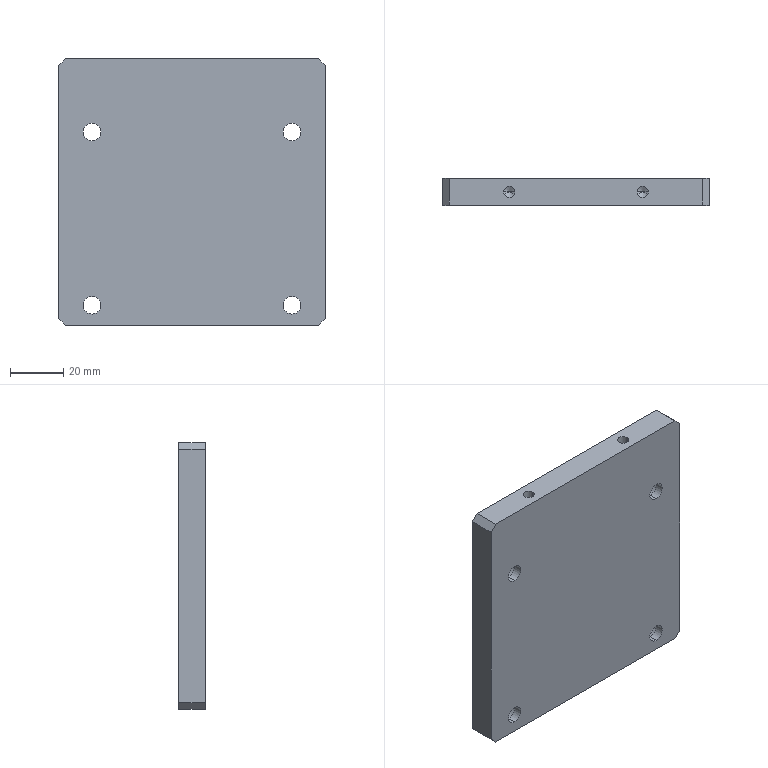Part | STEP file | Slide table mounting plate | 1 solid | 38 faces | box 100 x 10 x 100 mm | volume 96358 mm3 | cylinder 20 | plane 14 | cone 4 | commonest cylinder face diameters 6.6 x8 11 x8 4.2 x4